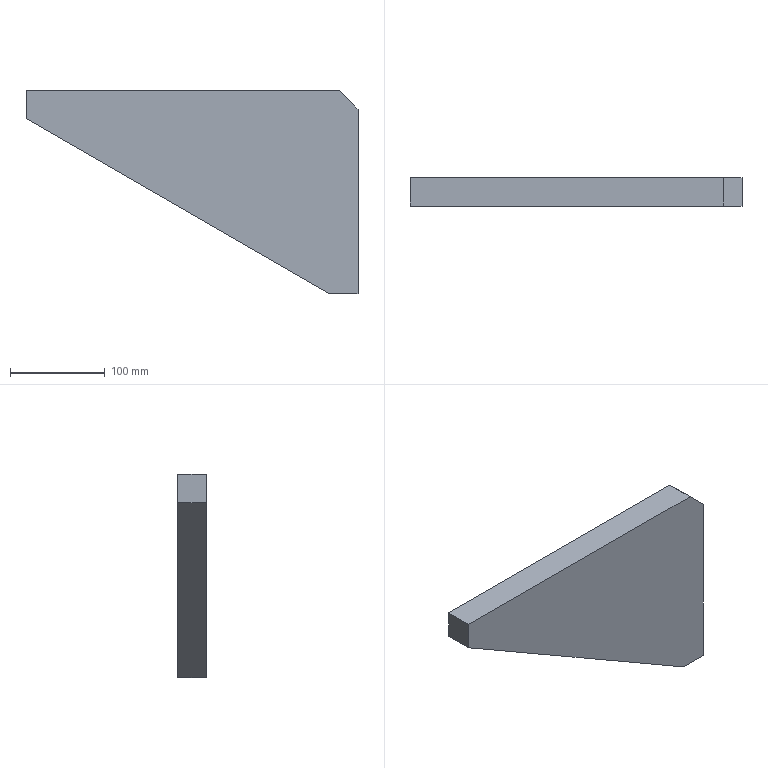Part | SolidWorks | features Extrusion 1 | 1 solid | 8 faces | box 350 x 30 x 214.752 mm | volume 1362087 mm3 | plane 8
STEP:
#1=CARTESIAN_POINT('',(0.,0.,194.752));
#2=VERTEX_POINT('',#1);
#3=CARTESIAN_POINT('',(0.,0.,0.));
#4=VERTEX_POINT('',#3);
#5=CARTESIAN_POINT('',(0.,0.,194.752));
#6=DIRECTION('',(0.,0.,-1.));
#7=VECTOR('',#6,1000.);
#8=LINE('',#5,#7);
#9=EDGE_CURVE('',#2,#4,#8,.T.);
#10=ORIENTED_EDGE('',*,*,#9,.T.);
#11=CARTESIAN_POINT('',(0.,30.,0.));
#12=VERTEX_POINT('',#11);
#13=CARTESIAN_POINT('',(0.,30.,0.));
#14=DIRECTION('',(0.,-1.,0.));
#15=VECTOR('',#14,1000.);
#16=LINE('',#13,#15);
#17=EDGE_CURVE('',#12,#4,#16,.T.);
#18=ORIENTED_EDGE('',*,*,#17,.F.);
#19=CARTESIAN_POINT('',(0.,30.,194.752));
#20=VERTEX_POINT('',#19);
#21=CARTESIAN_POINT('',(0.,30.,194.752));
#22=DIRECTION('',(0.,0.,-1.));
#23=VECTOR('',#22,1000.);
#24=LINE('',#21,#23);
#25=EDGE_CURVE('',#20,#12,#24,.T.);
#26=ORIENTED_EDGE('',*,*,#25,.F.);
#27=CARTESIAN_POINT('',(0.,30.,194.752));
#28=DIRECTION('',(0.,-1.,0.));
#29=VECTOR('',#28,1000.);
#30=LINE('',#27,#29);
#31=EDGE_CURVE('',#20,#2,#30,.T.);
#32=ORIENTED_EDGE('',*,*,#31,.T.);
#33=EDGE_LOOP('',(#10,#18,#26,#32));
#34=FACE_OUTER_BOUND('',#33,.T.);
#35=CARTESIAN_POINT('',(0.,30.,194.752));
#36=DIRECTION('',(-1.,0.,0.));
#37=DIRECTION('',(0.,0.,1.));
#38=AXIS2_PLACEMENT_3D('',#35,#36,#37);
#39=PLANE('',#38);
#40=ADVANCED_FACE('',(#34),#39,.F.);
#41=CARTESIAN_POINT('',(-30.,0.,0.));
#42=VERTEX_POINT('',#41);
#43=CARTESIAN_POINT('',(0.,0.,0.));
#44=DIRECTION('',(-1.,0.,0.));
#45=VECTOR('',#44,1000.);
#46=LINE('',#43,#45);
#47=EDGE_CURVE('',#4,#42,#46,.T.);
#48=ORIENTED_EDGE('',*,*,#47,.T.);
#49=CARTESIAN_POINT('',(-30.,30.,0.));
#50=VERTEX_POINT('',#49);
#51=CARTESIAN_POINT('',(-30.,30.,0.));
#52=DIRECTION('',(0.,-1.,0.));
#53=VECTOR('',#52,1000.);
#54=LINE('',#51,#53);
#55=EDGE_CURVE('',#50,#42,#54,.T.);
#56=ORIENTED_EDGE('',*,*,#55,.F.);
#57=CARTESIAN_POINT('',(0.,30.,0.));
#58=DIRECTION('',(-1.,0.,0.));
#59=VECTOR('',#58,1000.);
#60=LINE('',#57,#59);
#61=EDGE_CURVE('',#12,#50,#60,.T.);
#62=ORIENTED_EDGE('',*,*,#61,.F.);
#63=ORIENTED_EDGE('',*,*,#17,.T.);
#64=EDGE_LOOP('',(#48,#56,#62,#63));
#65=FACE_OUTER_BOUND('',#64,.T.);
#66=CARTESIAN_POINT('',(0.,30.,0.));
#67=DIRECTION('',(0.,0.,1.));
#68=DIRECTION('',(1.,0.,0.));
#69=AXIS2_PLACEMENT_3D('',#66,#67,#68);
#70=PLANE('',#69);
#71=ADVANCED_FACE('',(#65),#70,.F.);
#72=CARTESIAN_POINT('',(-350.,0.,184.752));
#73=VERTEX_POINT('',#72);
#74=CARTESIAN_POINT('',(-30.,0.,0.));
#75=DIRECTION('',(-0.866,0.,0.5));
#76=VECTOR('',#75,1000.);
#77=LINE('',#74,#76);
#78=EDGE_CURVE('',#42,#73,#77,.T.);
#79=ORIENTED_EDGE('',*,*,#78,.T.);
#80=CARTESIAN_POINT('',(-350.,30.,184.752));
#81=VERTEX_POINT('',#80);
#82=CARTESIAN_POINT('',(-350.,30.,184.752));
#83=DIRECTION('',(0.,-1.,0.));
#84=VECTOR('',#83,1000.);
#85=LINE('',#82,#84);
#86=EDGE_CURVE('',#81,#73,#85,.T.);
#87=ORIENTED_EDGE('',*,*,#86,.F.);
#88=CARTESIAN_POINT('',(-30.,30.,0.));
#89=DIRECTION('',(-0.866,0.,0.5));
#90=VECTOR('',#89,1000.);
#91=LINE('',#88,#90);
#92=EDGE_CURVE('',#50,#81,#91,.T.);
#93=ORIENTED_EDGE('',*,*,#92,.F.);
#94=ORIENTED_EDGE('',*,*,#55,.T.);
#95=EDGE_LOOP('',(#79,#87,#93,#94));
#96=FACE_OUTER_BOUND('',#95,.T.);
#97=CARTESIAN_POINT('',(-30.,30.,0.));
#98=DIRECTION('',(0.5,0.,0.866));
#99=DIRECTION('',(0.866,0.,-0.5));
#100=AXIS2_PLACEMENT_3D('',#97,#98,#99);
#101=PLANE('',#100);
#102=ADVANCED_FACE('',(#96),#101,.F.);
#103=CARTESIAN_POINT('',(-350.,0.,214.752));
#104=VERTEX_POINT('',#103);
#105=CARTESIAN_POINT('',(-350.,0.,184.752));
#106=DIRECTION('',(0.,0.,1.));
#107=VECTOR('',#106,1000.);
#108=LINE('',#105,#107);
#109=EDGE_CURVE('',#73,#104,#108,.T.);
#110=ORIENTED_EDGE('',*,*,#109,.T.);
#111=CARTESIAN_POINT('',(-350.,30.,214.752));
#112=VERTEX_POINT('',#111);
#113=CARTESIAN_POINT('',(-350.,30.,214.752));
#114=DIRECTION('',(0.,-1.,0.));
#115=VECTOR('',#114,1000.);
#116=LINE('',#113,#115);
#117=EDGE_CURVE('',#112,#104,#116,.T.);
#118=ORIENTED_EDGE('',*,*,#117,.F.);
#119=CARTESIAN_POINT('',(-350.,30.,184.752));
#120=DIRECTION('',(0.,0.,1.));
#121=VECTOR('',#120,1000.);
#122=LINE('',#119,#121);
#123=EDGE_CURVE('',#81,#112,#122,.T.);
#124=ORIENTED_EDGE('',*,*,#123,.F.);
#125=ORIENTED_EDGE('',*,*,#86,.T.);
#126=EDGE_LOOP('',(#110,#118,#124,#125));
#127=FACE_OUTER_BOUND('',#126,.T.);
#128=CARTESIAN_POINT('',(-350.,30.,184.752));
#129=DIRECTION('',(1.,0.,0.));
#130=DIRECTION('',(0.,0.,-1.));
#131=AXIS2_PLACEMENT_3D('',#128,#129,#130);
#132=PLANE('',#131);
#133=ADVANCED_FACE('',(#127),#132,.F.);
#134=CARTESIAN_POINT('',(-20.,0.,214.752));
#135=VERTEX_POINT('',#134);
#136=CARTESIAN_POINT('',(-350.,0.,214.752));
#137=DIRECTION('',(1.,0.,0.));
#138=VECTOR('',#137,1000.);
#139=LINE('',#136,#138);
#140=EDGE_CURVE('',#104,#135,#139,.T.);
#141=ORIENTED_EDGE('',*,*,#140,.T.);
#142=CARTESIAN_POINT('',(-20.,30.,214.752));
#143=VERTEX_POINT('',#142);
#144=CARTESIAN_POINT('',(-20.,30.,214.752));
#145=DIRECTION('',(0.,-1.,0.));
#146=VECTOR('',#145,1000.);
#147=LINE('',#144,#146);
#148=EDGE_CURVE('',#143,#135,#147,.T.);
#149=ORIENTED_EDGE('',*,*,#148,.F.);
#150=CARTESIAN_POINT('',(-350.,30.,214.752));
#151=DIRECTION('',(1.,0.,0.));
#152=VECTOR('',#151,1000.);
#153=LINE('',#150,#152);
#154=EDGE_CURVE('',#112,#143,#153,.T.);
#155=ORIENTED_EDGE('',*,*,#154,.F.);
#156=ORIENTED_EDGE('',*,*,#117,.T.);
#157=EDGE_LOOP('',(#141,#149,#155,#156));
#158=FACE_OUTER_BOUND('',#157,.T.);
#159=CARTESIAN_POINT('',(-350.,30.,214.752));
#160=DIRECTION('',(0.,0.,-1.));
#161=DIRECTION('',(-1.,0.,0.));
#162=AXIS2_PLACEMENT_3D('',#159,#160,#161);
#163=PLANE('',#162);
#164=ADVANCED_FACE('',(#158),#163,.F.);
#165=CARTESIAN_POINT('',(-20.,0.,214.752));
#166=DIRECTION('',(0.7071,0.,-0.7071));
#167=VECTOR('',#166,1000.);
#168=LINE('',#165,#167);
#169=EDGE_CURVE('',#135,#2,#168,.T.);
#170=ORIENTED_EDGE('',*,*,#169,.T.);
#171=ORIENTED_EDGE('',*,*,#31,.F.);
#172=CARTESIAN_POINT('',(-20.,30.,214.752));
#173=DIRECTION('',(0.7071,0.,-0.7071));
#174=VECTOR('',#173,1000.);
#175=LINE('',#172,#174);
#176=EDGE_CURVE('',#143,#20,#175,.T.);
#177=ORIENTED_EDGE('',*,*,#176,.F.);
#178=ORIENTED_EDGE('',*,*,#148,.T.);
#179=EDGE_LOOP('',(#170,#171,#177,#178));
#180=FACE_OUTER_BOUND('',#179,.T.);
#181=CARTESIAN_POINT('',(-20.,30.,214.752));
#182=DIRECTION('',(-0.7071,0.,-0.7071));
#183=DIRECTION('',(-0.7071,0.,0.7071));
#184=AXIS2_PLACEMENT_3D('',#181,#182,#183);
#185=PLANE('',#184);
#186=ADVANCED_FACE('',(#180),#185,.F.);
#187=ORIENTED_EDGE('',*,*,#25,.T.);
#188=ORIENTED_EDGE('',*,*,#61,.T.);
#189=ORIENTED_EDGE('',*,*,#92,.T.);
#190=ORIENTED_EDGE('',*,*,#123,.T.);
#191=ORIENTED_EDGE('',*,*,#154,.T.);
#192=ORIENTED_EDGE('',*,*,#176,.T.);
#193=EDGE_LOOP('',(#187,#188,#189,#190,#191,#192));
#194=FACE_OUTER_BOUND('',#193,.T.);
#195=CARTESIAN_POINT('',(0.,30.,0.));
#196=DIRECTION('',(0.,1.,0.));
#197=DIRECTION('',(0.,0.,1.));
#198=AXIS2_PLACEMENT_3D('',#195,#196,#197);
#199=PLANE('',#198);
#200=ADVANCED_FACE('',(#194),#199,.T.);
#201=ORIENTED_EDGE('',*,*,#9,.F.);
#202=ORIENTED_EDGE('',*,*,#169,.F.);
#203=ORIENTED_EDGE('',*,*,#140,.F.);
#204=ORIENTED_EDGE('',*,*,#109,.F.);
#205=ORIENTED_EDGE('',*,*,#78,.F.);
#206=ORIENTED_EDGE('',*,*,#47,.F.);
#207=EDGE_LOOP('',(#201,#202,#203,#204,#205,#206));
#208=FACE_OUTER_BOUND('',#207,.T.);
#209=CARTESIAN_POINT('',(0.,0.,0.));
#210=DIRECTION('',(0.,1.,0.));
#211=DIRECTION('',(0.,0.,1.));
#212=AXIS2_PLACEMENT_3D('',#209,#210,#211);
#213=PLANE('',#212);
#214=ADVANCED_FACE('',(#208),#213,.F.);
#215=CLOSED_SHELL('',(#40,#71,#102,#133,#164,#186,#200,#214));
#216=MANIFOLD_SOLID_BREP('',#215);
#217=CARTESIAN_POINT('',(0.,0.,0.));
#218=DIRECTION('',(0.,0.,1.));
#219=DIRECTION('',(1.,0.,0.));
#220=AXIS2_PLACEMENT_3D('',#217,#218,#219);
#221=(LENGTH_UNIT()NAMED_UNIT(*)SI_UNIT(.MILLI.,.METRE.));
#222=UNCERTAINTY_MEASURE_WITH_UNIT(LENGTH_MEASURE(0.00001),#221,'','');
#223=(NAMED_UNIT(*)PLANE_ANGLE_UNIT()SI_UNIT($,.RADIAN.));
#224=(NAMED_UNIT(*)SI_UNIT($,.STERADIAN.)SOLID_ANGLE_UNIT());
#225=(GEOMETRIC_REPRESENTATION_CONTEXT(3)GLOBAL_UNCERTAINTY_ASSIGNED_CONTEXT((#222))GLOBAL_UNIT_ASSIGNED_CONTEXT((#221,#223,#224))REPRESENTATION_CONTEXT('',''));
#226=ADVANCED_BREP_SHAPE_REPRESENTATION('',(#216,#220),#225);